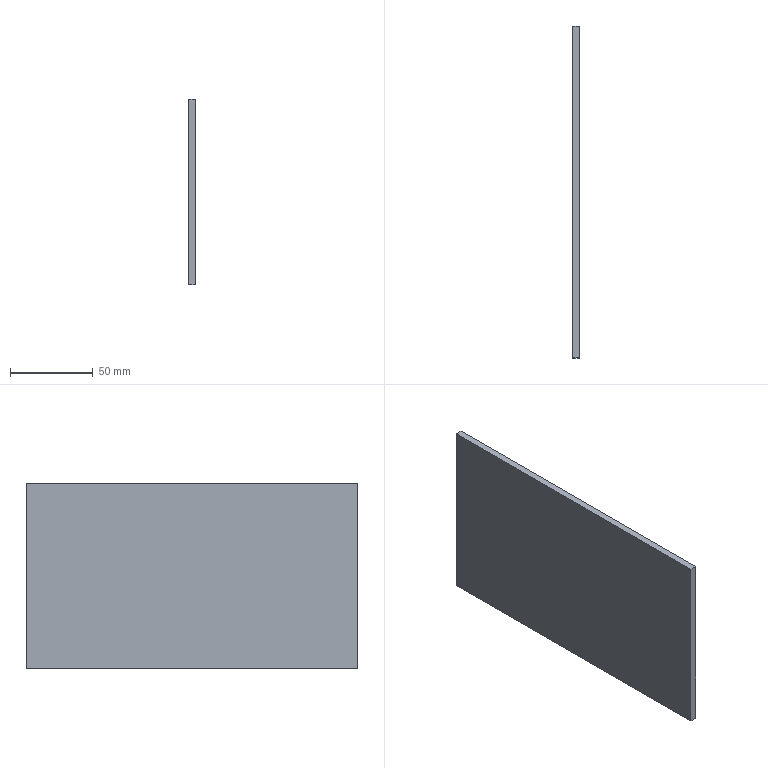Part | SolidWorks | features Extrusion 1 | 1 solid | 6 faces | box 4 x 200 x 112 mm | volume 89600 mm3 | plane 6
STEP:
#1=CARTESIAN_POINT('',(0.,200.,0.));
#2=VERTEX_POINT('',#1);
#3=CARTESIAN_POINT('',(0.,0.,0.));
#4=VERTEX_POINT('',#3);
#5=CARTESIAN_POINT('',(0.,0.,0.));
#6=DIRECTION('',(0.,-1.,0.));
#7=VECTOR('',#6,1000.);
#8=LINE('',#5,#7);
#9=EDGE_CURVE('',#2,#4,#8,.T.);
#10=ORIENTED_EDGE('',*,*,#9,.T.);
#11=CARTESIAN_POINT('',(4.,0.,0.));
#12=VERTEX_POINT('',#11);
#13=CARTESIAN_POINT('',(4.,0.,0.));
#14=DIRECTION('',(-1.,0.,0.));
#15=VECTOR('',#14,1000.);
#16=LINE('',#13,#15);
#17=EDGE_CURVE('',#12,#4,#16,.T.);
#18=ORIENTED_EDGE('',*,*,#17,.F.);
#19=CARTESIAN_POINT('',(4.,200.,0.));
#20=VERTEX_POINT('',#19);
#21=CARTESIAN_POINT('',(4.,0.,0.));
#22=DIRECTION('',(0.,-1.,0.));
#23=VECTOR('',#22,1000.);
#24=LINE('',#21,#23);
#25=EDGE_CURVE('',#20,#12,#24,.T.);
#26=ORIENTED_EDGE('',*,*,#25,.F.);
#27=CARTESIAN_POINT('',(4.,200.,0.));
#28=DIRECTION('',(-1.,0.,0.));
#29=VECTOR('',#28,1000.);
#30=LINE('',#27,#29);
#31=EDGE_CURVE('',#20,#2,#30,.T.);
#32=ORIENTED_EDGE('',*,*,#31,.T.);
#33=EDGE_LOOP('',(#10,#18,#26,#32));
#34=FACE_OUTER_BOUND('',#33,.T.);
#35=CARTESIAN_POINT('',(4.,0.,0.));
#36=DIRECTION('',(0.,0.,-1.));
#37=DIRECTION('',(-1.,0.,0.));
#38=AXIS2_PLACEMENT_3D('',#35,#36,#37);
#39=PLANE('',#38);
#40=ADVANCED_FACE('',(#34),#39,.F.);
#41=CARTESIAN_POINT('',(0.,0.,-112.));
#42=VERTEX_POINT('',#41);
#43=CARTESIAN_POINT('',(0.,0.,0.));
#44=DIRECTION('',(0.,0.,-1.));
#45=VECTOR('',#44,1000.);
#46=LINE('',#43,#45);
#47=EDGE_CURVE('',#4,#42,#46,.T.);
#48=ORIENTED_EDGE('',*,*,#47,.T.);
#49=CARTESIAN_POINT('',(4.,0.,-112.));
#50=VERTEX_POINT('',#49);
#51=CARTESIAN_POINT('',(4.,0.,-112.));
#52=DIRECTION('',(-1.,0.,0.));
#53=VECTOR('',#52,1000.);
#54=LINE('',#51,#53);
#55=EDGE_CURVE('',#50,#42,#54,.T.);
#56=ORIENTED_EDGE('',*,*,#55,.F.);
#57=CARTESIAN_POINT('',(4.,0.,0.));
#58=DIRECTION('',(0.,0.,-1.));
#59=VECTOR('',#58,1000.);
#60=LINE('',#57,#59);
#61=EDGE_CURVE('',#12,#50,#60,.T.);
#62=ORIENTED_EDGE('',*,*,#61,.F.);
#63=ORIENTED_EDGE('',*,*,#17,.T.);
#64=EDGE_LOOP('',(#48,#56,#62,#63));
#65=FACE_OUTER_BOUND('',#64,.T.);
#66=CARTESIAN_POINT('',(4.,0.,0.));
#67=DIRECTION('',(0.,1.,0.));
#68=DIRECTION('',(0.,0.,1.));
#69=AXIS2_PLACEMENT_3D('',#66,#67,#68);
#70=PLANE('',#69);
#71=ADVANCED_FACE('',(#65),#70,.F.);
#72=CARTESIAN_POINT('',(0.,200.,-112.));
#73=VERTEX_POINT('',#72);
#74=CARTESIAN_POINT('',(0.,0.,-112.));
#75=DIRECTION('',(0.,1.,0.));
#76=VECTOR('',#75,1000.);
#77=LINE('',#74,#76);
#78=EDGE_CURVE('',#42,#73,#77,.T.);
#79=ORIENTED_EDGE('',*,*,#78,.T.);
#80=CARTESIAN_POINT('',(4.,200.,-112.));
#81=VERTEX_POINT('',#80);
#82=CARTESIAN_POINT('',(4.,200.,-112.));
#83=DIRECTION('',(-1.,0.,0.));
#84=VECTOR('',#83,1000.);
#85=LINE('',#82,#84);
#86=EDGE_CURVE('',#81,#73,#85,.T.);
#87=ORIENTED_EDGE('',*,*,#86,.F.);
#88=CARTESIAN_POINT('',(4.,0.,-112.));
#89=DIRECTION('',(0.,1.,0.));
#90=VECTOR('',#89,1000.);
#91=LINE('',#88,#90);
#92=EDGE_CURVE('',#50,#81,#91,.T.);
#93=ORIENTED_EDGE('',*,*,#92,.F.);
#94=ORIENTED_EDGE('',*,*,#55,.T.);
#95=EDGE_LOOP('',(#79,#87,#93,#94));
#96=FACE_OUTER_BOUND('',#95,.T.);
#97=CARTESIAN_POINT('',(4.,0.,-112.));
#98=DIRECTION('',(0.,0.,1.));
#99=DIRECTION('',(1.,0.,0.));
#100=AXIS2_PLACEMENT_3D('',#97,#98,#99);
#101=PLANE('',#100);
#102=ADVANCED_FACE('',(#96),#101,.F.);
#103=CARTESIAN_POINT('',(0.,200.,0.));
#104=DIRECTION('',(0.,0.,1.));
#105=VECTOR('',#104,1000.);
#106=LINE('',#103,#105);
#107=EDGE_CURVE('',#73,#2,#106,.T.);
#108=ORIENTED_EDGE('',*,*,#107,.T.);
#109=ORIENTED_EDGE('',*,*,#31,.F.);
#110=CARTESIAN_POINT('',(4.,200.,0.));
#111=DIRECTION('',(0.,0.,1.));
#112=VECTOR('',#111,1000.);
#113=LINE('',#110,#112);
#114=EDGE_CURVE('',#81,#20,#113,.T.);
#115=ORIENTED_EDGE('',*,*,#114,.F.);
#116=ORIENTED_EDGE('',*,*,#86,.T.);
#117=EDGE_LOOP('',(#108,#109,#115,#116));
#118=FACE_OUTER_BOUND('',#117,.T.);
#119=CARTESIAN_POINT('',(4.,200.,0.));
#120=DIRECTION('',(0.,-1.,0.));
#121=DIRECTION('',(0.,0.,-1.));
#122=AXIS2_PLACEMENT_3D('',#119,#120,#121);
#123=PLANE('',#122);
#124=ADVANCED_FACE('',(#118),#123,.F.);
#125=ORIENTED_EDGE('',*,*,#25,.T.);
#126=ORIENTED_EDGE('',*,*,#61,.T.);
#127=ORIENTED_EDGE('',*,*,#92,.T.);
#128=ORIENTED_EDGE('',*,*,#114,.T.);
#129=EDGE_LOOP('',(#125,#126,#127,#128));
#130=FACE_OUTER_BOUND('',#129,.T.);
#131=CARTESIAN_POINT('',(4.,0.,0.));
#132=DIRECTION('',(-1.,0.,0.));
#133=DIRECTION('',(0.,0.,1.));
#134=AXIS2_PLACEMENT_3D('',#131,#132,#133);
#135=PLANE('',#134);
#136=ADVANCED_FACE('',(#130),#135,.F.);
#137=ORIENTED_EDGE('',*,*,#9,.F.);
#138=ORIENTED_EDGE('',*,*,#107,.F.);
#139=ORIENTED_EDGE('',*,*,#78,.F.);
#140=ORIENTED_EDGE('',*,*,#47,.F.);
#141=EDGE_LOOP('',(#137,#138,#139,#140));
#142=FACE_OUTER_BOUND('',#141,.T.);
#143=CARTESIAN_POINT('',(0.,0.,0.));
#144=DIRECTION('',(-1.,0.,0.));
#145=DIRECTION('',(0.,0.,1.));
#146=AXIS2_PLACEMENT_3D('',#143,#144,#145);
#147=PLANE('',#146);
#148=ADVANCED_FACE('',(#142),#147,.T.);
#149=CLOSED_SHELL('',(#40,#71,#102,#124,#136,#148));
#150=MANIFOLD_SOLID_BREP('',#149);
#151=CARTESIAN_POINT('',(0.,0.,0.));
#152=DIRECTION('',(0.,0.,1.));
#153=DIRECTION('',(1.,0.,0.));
#154=AXIS2_PLACEMENT_3D('',#151,#152,#153);
#155=(LENGTH_UNIT()NAMED_UNIT(*)SI_UNIT(.MILLI.,.METRE.));
#156=UNCERTAINTY_MEASURE_WITH_UNIT(LENGTH_MEASURE(0.00001),#155,'','');
#157=(NAMED_UNIT(*)PLANE_ANGLE_UNIT()SI_UNIT($,.RADIAN.));
#158=(NAMED_UNIT(*)SI_UNIT($,.STERADIAN.)SOLID_ANGLE_UNIT());
#159=(GEOMETRIC_REPRESENTATION_CONTEXT(3)GLOBAL_UNCERTAINTY_ASSIGNED_CONTEXT((#156))GLOBAL_UNIT_ASSIGNED_CONTEXT((#155,#157,#158))REPRESENTATION_CONTEXT('',''));
#160=ADVANCED_BREP_SHAPE_REPRESENTATION('',(#150,#154),#159);